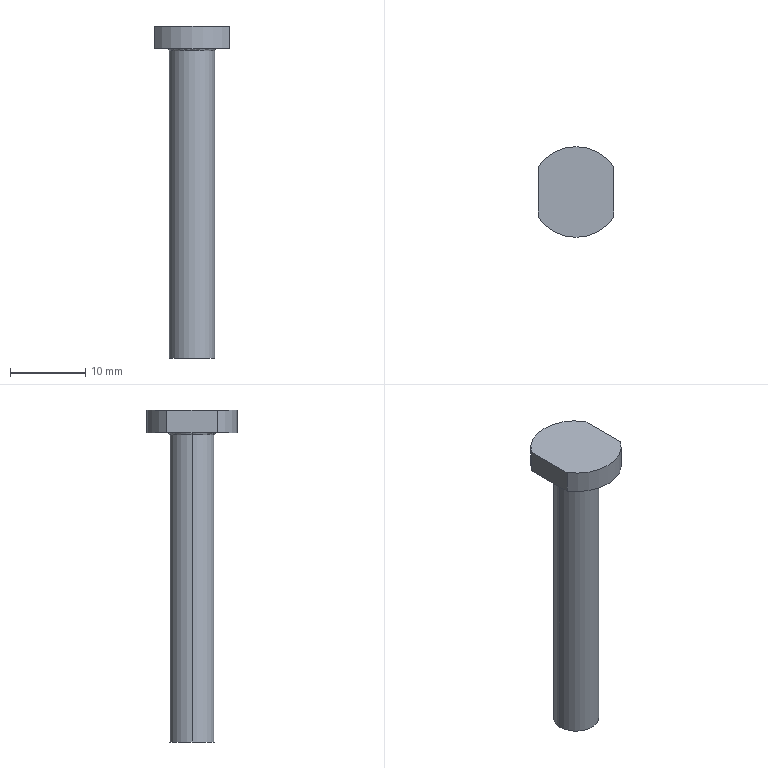Part | STEP file | Guide post | 1 solid | 14 faces | box 10 x 12 x 44 mm | volume 1435 mm3 | cylinder 6 | plane 6 | spline 2 | commonest cylinder face diameters 2.5 x2 6 x2 12 x2